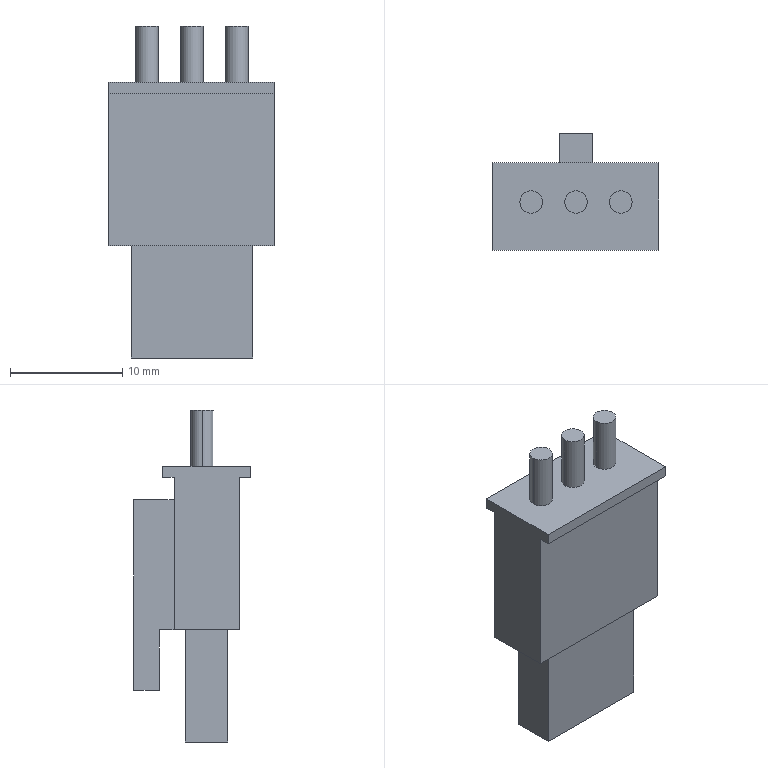Part | STEP file | ELP_03V | 1 solid | 30 faces | box 14.8 x 10.4 x 29.6 mm | volume 1903 mm3 | plane 24 | cylinder 6 | commonest cylinder face diameters 2 x6